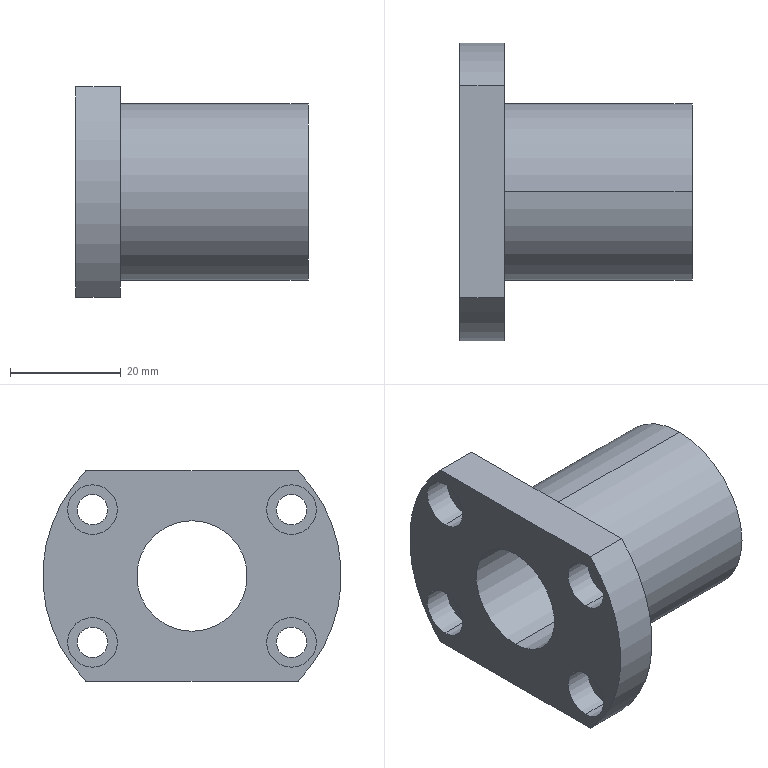Part | SolidWorks | features BaseBody 1 | 1 solid | 31 faces | box 42 x 54 x 38 mm | volume 27513 mm3 | cylinder 22 | plane 9 | commonest cylinder face diameters 5.5 x8 9 x8 20 x2 32 x2 54 x2
STEP:
#1=CARTESIAN_POINT('',(42.,0.,16.));
#2=VERTEX_POINT('',#1);
#3=CARTESIAN_POINT('',(42.,0.,-16.));
#4=VERTEX_POINT('',#3);
#5=CARTESIAN_POINT('',(42.,0.,0.));
#6=DIRECTION('',(-1.,0.,0.));
#7=DIRECTION('',(0.,0.,1.));
#8=AXIS2_PLACEMENT_3D('',#5,#6,#7);
#9=CIRCLE('',#8,16.);
#10=EDGE_CURVE('',#2,#4,#9,.T.);
#11=ORIENTED_EDGE('',*,*,#10,.T.);
#12=CARTESIAN_POINT('',(8.,0.,-16.));
#13=VERTEX_POINT('',#12);
#14=CARTESIAN_POINT('',(0.,0.,-16.));
#15=DIRECTION('',(-1.,0.,0.));
#16=VECTOR('',#15,1000.);
#17=LINE('',#14,#16);
#18=EDGE_CURVE('',#4,#13,#17,.T.);
#19=ORIENTED_EDGE('',*,*,#18,.T.);
#20=CARTESIAN_POINT('',(8.,0.,16.));
#21=VERTEX_POINT('',#20);
#22=CARTESIAN_POINT('',(8.,0.,0.));
#23=DIRECTION('',(1.,0.,0.));
#24=DIRECTION('',(0.,0.,1.));
#25=AXIS2_PLACEMENT_3D('',#22,#23,#24);
#26=CIRCLE('',#25,16.);
#27=EDGE_CURVE('',#13,#21,#26,.T.);
#28=ORIENTED_EDGE('',*,*,#27,.T.);
#29=CARTESIAN_POINT('',(0.,0.,16.));
#30=DIRECTION('',(-1.,0.,0.));
#31=VECTOR('',#30,1000.);
#32=LINE('',#29,#31);
#33=EDGE_CURVE('',#2,#21,#32,.T.);
#34=ORIENTED_EDGE('',*,*,#33,.F.);
#35=EDGE_LOOP('',(#11,#19,#28,#34));
#36=FACE_OUTER_BOUND('',#35,.T.);
#37=CARTESIAN_POINT('',(0.,0.,0.));
#38=DIRECTION('',(-1.,0.,0.));
#39=DIRECTION('',(0.,0.,1.));
#40=AXIS2_PLACEMENT_3D('',#37,#38,#39);
#41=CYLINDRICAL_SURFACE('',#40,16.);
#42=ADVANCED_FACE('',(#36),#41,.T.);
#43=CARTESIAN_POINT('',(8.,18.,14.75));
#44=VERTEX_POINT('',#43);
#45=CARTESIAN_POINT('',(8.,18.,9.25));
#46=VERTEX_POINT('',#45);
#47=CARTESIAN_POINT('',(8.,18.,12.));
#48=DIRECTION('',(1.,0.,0.));
#49=DIRECTION('',(0.,0.,1.));
#50=AXIS2_PLACEMENT_3D('',#47,#48,#49);
#51=CIRCLE('',#50,2.75);
#52=EDGE_CURVE('',#44,#46,#51,.T.);
#53=ORIENTED_EDGE('',*,*,#52,.T.);
#54=CARTESIAN_POINT('',(5.1,18.,9.25));
#55=VERTEX_POINT('',#54);
#56=CARTESIAN_POINT('',(42.001,18.,9.25));
#57=DIRECTION('',(-1.,0.,0.));
#58=VECTOR('',#57,1000.);
#59=LINE('',#56,#58);
#60=EDGE_CURVE('',#46,#55,#59,.T.);
#61=ORIENTED_EDGE('',*,*,#60,.T.);
#62=CARTESIAN_POINT('',(5.1,18.,14.75));
#63=VERTEX_POINT('',#62);
#64=CARTESIAN_POINT('',(5.1,18.,12.));
#65=DIRECTION('',(1.,0.,0.));
#66=DIRECTION('',(0.,0.,1.));
#67=AXIS2_PLACEMENT_3D('',#64,#65,#66);
#68=CIRCLE('',#67,2.75);
#69=EDGE_CURVE('',#63,#55,#68,.T.);
#70=ORIENTED_EDGE('',*,*,#69,.F.);
#71=CARTESIAN_POINT('',(42.001,18.,14.75));
#72=DIRECTION('',(-1.,0.,0.));
#73=VECTOR('',#72,1000.);
#74=LINE('',#71,#73);
#75=EDGE_CURVE('',#44,#63,#74,.T.);
#76=ORIENTED_EDGE('',*,*,#75,.F.);
#77=EDGE_LOOP('',(#53,#61,#70,#76));
#78=FACE_OUTER_BOUND('',#77,.T.);
#79=CARTESIAN_POINT('',(42.001,18.,12.));
#80=DIRECTION('',(-1.,0.,0.));
#81=DIRECTION('',(0.,0.,1.));
#82=AXIS2_PLACEMENT_3D('',#79,#80,#81);
#83=CYLINDRICAL_SURFACE('',#82,2.75);
#84=ADVANCED_FACE('',(#78),#83,.F.);
#85=CARTESIAN_POINT('',(8.,18.,-9.25));
#86=VERTEX_POINT('',#85);
#87=CARTESIAN_POINT('',(8.,18.,-14.75));
#88=VERTEX_POINT('',#87);
#89=CARTESIAN_POINT('',(8.,18.,-12.));
#90=DIRECTION('',(1.,0.,0.));
#91=DIRECTION('',(0.,0.,1.));
#92=AXIS2_PLACEMENT_3D('',#89,#90,#91);
#93=CIRCLE('',#92,2.75);
#94=EDGE_CURVE('',#86,#88,#93,.T.);
#95=ORIENTED_EDGE('',*,*,#94,.T.);
#96=CARTESIAN_POINT('',(5.1,18.,-14.75));
#97=VERTEX_POINT('',#96);
#98=CARTESIAN_POINT('',(42.001,18.,-14.75));
#99=DIRECTION('',(-1.,0.,0.));
#100=VECTOR('',#99,1000.);
#101=LINE('',#98,#100);
#102=EDGE_CURVE('',#88,#97,#101,.T.);
#103=ORIENTED_EDGE('',*,*,#102,.T.);
#104=CARTESIAN_POINT('',(5.1,18.,-9.25));
#105=VERTEX_POINT('',#104);
#106=CARTESIAN_POINT('',(5.1,18.,-12.));
#107=DIRECTION('',(1.,0.,0.));
#108=DIRECTION('',(0.,0.,1.));
#109=AXIS2_PLACEMENT_3D('',#106,#107,#108);
#110=CIRCLE('',#109,2.75);
#111=EDGE_CURVE('',#105,#97,#110,.T.);
#112=ORIENTED_EDGE('',*,*,#111,.F.);
#113=CARTESIAN_POINT('',(42.001,18.,-9.25));
#114=DIRECTION('',(-1.,0.,0.));
#115=VECTOR('',#114,1000.);
#116=LINE('',#113,#115);
#117=EDGE_CURVE('',#86,#105,#116,.T.);
#118=ORIENTED_EDGE('',*,*,#117,.F.);
#119=EDGE_LOOP('',(#95,#103,#112,#118));
#120=FACE_OUTER_BOUND('',#119,.T.);
#121=CARTESIAN_POINT('',(42.001,18.,-12.));
#122=DIRECTION('',(-1.,0.,0.));
#123=DIRECTION('',(0.,0.,1.));
#124=AXIS2_PLACEMENT_3D('',#121,#122,#123);
#125=CYLINDRICAL_SURFACE('',#124,2.75);
#126=ADVANCED_FACE('',(#120),#125,.F.);
#127=CARTESIAN_POINT('',(8.,-18.,-9.25));
#128=VERTEX_POINT('',#127);
#129=CARTESIAN_POINT('',(8.,-18.,-14.75));
#130=VERTEX_POINT('',#129);
#131=CARTESIAN_POINT('',(8.,-18.,-12.));
#132=DIRECTION('',(1.,0.,0.));
#133=DIRECTION('',(0.,0.,1.));
#134=AXIS2_PLACEMENT_3D('',#131,#132,#133);
#135=CIRCLE('',#134,2.75);
#136=EDGE_CURVE('',#128,#130,#135,.T.);
#137=ORIENTED_EDGE('',*,*,#136,.T.);
#138=CARTESIAN_POINT('',(5.1,-18.,-14.75));
#139=VERTEX_POINT('',#138);
#140=CARTESIAN_POINT('',(42.001,-18.,-14.75));
#141=DIRECTION('',(-1.,0.,0.));
#142=VECTOR('',#141,1000.);
#143=LINE('',#140,#142);
#144=EDGE_CURVE('',#130,#139,#143,.T.);
#145=ORIENTED_EDGE('',*,*,#144,.T.);
#146=CARTESIAN_POINT('',(5.1,-18.,-9.25));
#147=VERTEX_POINT('',#146);
#148=CARTESIAN_POINT('',(5.1,-18.,-12.));
#149=DIRECTION('',(1.,0.,0.));
#150=DIRECTION('',(0.,0.,1.));
#151=AXIS2_PLACEMENT_3D('',#148,#149,#150);
#152=CIRCLE('',#151,2.75);
#153=EDGE_CURVE('',#147,#139,#152,.T.);
#154=ORIENTED_EDGE('',*,*,#153,.F.);
#155=CARTESIAN_POINT('',(42.001,-18.,-9.25));
#156=DIRECTION('',(-1.,0.,0.));
#157=VECTOR('',#156,1000.);
#158=LINE('',#155,#157);
#159=EDGE_CURVE('',#128,#147,#158,.T.);
#160=ORIENTED_EDGE('',*,*,#159,.F.);
#161=EDGE_LOOP('',(#137,#145,#154,#160));
#162=FACE_OUTER_BOUND('',#161,.T.);
#163=CARTESIAN_POINT('',(42.001,-18.,-12.));
#164=DIRECTION('',(-1.,0.,0.));
#165=DIRECTION('',(0.,0.,1.));
#166=AXIS2_PLACEMENT_3D('',#163,#164,#165);
#167=CYLINDRICAL_SURFACE('',#166,2.75);
#168=ADVANCED_FACE('',(#162),#167,.F.);
#169=CARTESIAN_POINT('',(8.,-18.,14.75));
#170=VERTEX_POINT('',#169);
#171=CARTESIAN_POINT('',(8.,-18.,9.25));
#172=VERTEX_POINT('',#171);
#173=CARTESIAN_POINT('',(8.,-18.,12.));
#174=DIRECTION('',(1.,0.,0.));
#175=DIRECTION('',(0.,0.,1.));
#176=AXIS2_PLACEMENT_3D('',#173,#174,#175);
#177=CIRCLE('',#176,2.75);
#178=EDGE_CURVE('',#170,#172,#177,.T.);
#179=ORIENTED_EDGE('',*,*,#178,.T.);
#180=CARTESIAN_POINT('',(5.1,-18.,9.25));
#181=VERTEX_POINT('',#180);
#182=CARTESIAN_POINT('',(42.001,-18.,9.25));
#183=DIRECTION('',(-1.,0.,0.));
#184=VECTOR('',#183,1000.);
#185=LINE('',#182,#184);
#186=EDGE_CURVE('',#172,#181,#185,.T.);
#187=ORIENTED_EDGE('',*,*,#186,.T.);
#188=CARTESIAN_POINT('',(5.1,-18.,14.75));
#189=VERTEX_POINT('',#188);
#190=CARTESIAN_POINT('',(5.1,-18.,12.));
#191=DIRECTION('',(1.,0.,0.));
#192=DIRECTION('',(0.,0.,1.));
#193=AXIS2_PLACEMENT_3D('',#190,#191,#192);
#194=CIRCLE('',#193,2.75);
#195=EDGE_CURVE('',#189,#181,#194,.T.);
#196=ORIENTED_EDGE('',*,*,#195,.F.);
#197=CARTESIAN_POINT('',(42.001,-18.,14.75));
#198=DIRECTION('',(-1.,0.,0.));
#199=VECTOR('',#198,1000.);
#200=LINE('',#197,#199);
#201=EDGE_CURVE('',#170,#189,#200,.T.);
#202=ORIENTED_EDGE('',*,*,#201,.F.);
#203=EDGE_LOOP('',(#179,#187,#196,#202));
#204=FACE_OUTER_BOUND('',#203,.T.);
#205=CARTESIAN_POINT('',(42.001,-18.,12.));
#206=DIRECTION('',(-1.,0.,0.));
#207=DIRECTION('',(0.,0.,1.));
#208=AXIS2_PLACEMENT_3D('',#205,#206,#207);
#209=CYLINDRICAL_SURFACE('',#208,2.75);
#210=ADVANCED_FACE('',(#204),#209,.F.);
#211=CARTESIAN_POINT('',(42.,0.,10.));
#212=VERTEX_POINT('',#211);
#213=CARTESIAN_POINT('',(42.,0.,-10.));
#214=VERTEX_POINT('',#213);
#215=CARTESIAN_POINT('',(42.,0.,0.));
#216=DIRECTION('',(1.,0.,0.));
#217=DIRECTION('',(0.,0.,1.));
#218=AXIS2_PLACEMENT_3D('',#215,#216,#217);
#219=CIRCLE('',#218,10.);
#220=EDGE_CURVE('',#212,#214,#219,.T.);
#221=ORIENTED_EDGE('',*,*,#220,.T.);
#222=CARTESIAN_POINT('',(0.,0.,-10.));
#223=VERTEX_POINT('',#222);
#224=CARTESIAN_POINT('',(0.,0.,-10.));
#225=DIRECTION('',(-1.,0.,0.));
#226=VECTOR('',#225,1000.);
#227=LINE('',#224,#226);
#228=EDGE_CURVE('',#214,#223,#227,.T.);
#229=ORIENTED_EDGE('',*,*,#228,.T.);
#230=CARTESIAN_POINT('',(0.,0.,10.));
#231=VERTEX_POINT('',#230);
#232=CARTESIAN_POINT('',(0.,0.,0.));
#233=DIRECTION('',(1.,0.,0.));
#234=DIRECTION('',(0.,0.,1.));
#235=AXIS2_PLACEMENT_3D('',#232,#233,#234);
#236=CIRCLE('',#235,10.);
#237=EDGE_CURVE('',#231,#223,#236,.T.);
#238=ORIENTED_EDGE('',*,*,#237,.F.);
#239=CARTESIAN_POINT('',(0.,0.,10.));
#240=DIRECTION('',(-1.,0.,0.));
#241=VECTOR('',#240,1000.);
#242=LINE('',#239,#241);
#243=EDGE_CURVE('',#212,#231,#242,.T.);
#244=ORIENTED_EDGE('',*,*,#243,.F.);
#245=EDGE_LOOP('',(#221,#229,#238,#244));
#246=FACE_OUTER_BOUND('',#245,.T.);
#247=CARTESIAN_POINT('',(0.,0.,0.));
#248=DIRECTION('',(-1.,0.,0.));
#249=DIRECTION('',(0.,0.,1.));
#250=AXIS2_PLACEMENT_3D('',#247,#248,#249);
#251=CYLINDRICAL_SURFACE('',#250,10.);
#252=ADVANCED_FACE('',(#246),#251,.F.);
#253=CARTESIAN_POINT('',(5.1,18.,7.5));
#254=VERTEX_POINT('',#253);
#255=CARTESIAN_POINT('',(5.1,18.,16.5));
#256=VERTEX_POINT('',#255);
#257=CARTESIAN_POINT('',(5.1,18.,12.));
#258=DIRECTION('',(-1.,0.,0.));
#259=DIRECTION('',(0.,0.,1.));
#260=AXIS2_PLACEMENT_3D('',#257,#258,#259);
#261=CIRCLE('',#260,4.5);
#262=EDGE_CURVE('',#254,#256,#261,.T.);
#263=ORIENTED_EDGE('',*,*,#262,.F.);
#264=CARTESIAN_POINT('',(0.,18.,7.5));
#265=VERTEX_POINT('',#264);
#266=CARTESIAN_POINT('',(5.1,18.,7.5));
#267=DIRECTION('',(-1.,0.,0.));
#268=VECTOR('',#267,1000.);
#269=LINE('',#266,#268);
#270=EDGE_CURVE('',#254,#265,#269,.T.);
#271=ORIENTED_EDGE('',*,*,#270,.T.);
#272=CARTESIAN_POINT('',(0.,18.,16.5));
#273=VERTEX_POINT('',#272);
#274=CARTESIAN_POINT('',(0.,18.,12.));
#275=DIRECTION('',(-1.,0.,0.));
#276=DIRECTION('',(0.,0.,1.));
#277=AXIS2_PLACEMENT_3D('',#274,#275,#276);
#278=CIRCLE('',#277,4.5);
#279=EDGE_CURVE('',#265,#273,#278,.T.);
#280=ORIENTED_EDGE('',*,*,#279,.T.);
#281=CARTESIAN_POINT('',(5.1,18.,16.5));
#282=DIRECTION('',(-1.,0.,0.));
#283=VECTOR('',#282,1000.);
#284=LINE('',#281,#283);
#285=EDGE_CURVE('',#256,#273,#284,.T.);
#286=ORIENTED_EDGE('',*,*,#285,.F.);
#287=EDGE_LOOP('',(#263,#271,#280,#286));
#288=FACE_OUTER_BOUND('',#287,.T.);
#289=CARTESIAN_POINT('',(5.1,18.,12.));
#290=DIRECTION('',(-1.,0.,0.));
#291=DIRECTION('',(0.,0.,1.));
#292=AXIS2_PLACEMENT_3D('',#289,#290,#291);
#293=CYLINDRICAL_SURFACE('',#292,4.5);
#294=ADVANCED_FACE('',(#288),#293,.F.);
#295=CARTESIAN_POINT('',(5.1,18.,-16.5));
#296=VERTEX_POINT('',#295);
#297=CARTESIAN_POINT('',(5.1,18.,-7.5));
#298=VERTEX_POINT('',#297);
#299=CARTESIAN_POINT('',(5.1,18.,-12.));
#300=DIRECTION('',(-1.,0.,0.));
#301=DIRECTION('',(0.,0.,1.));
#302=AXIS2_PLACEMENT_3D('',#299,#300,#301);
#303=CIRCLE('',#302,4.5);
#304=EDGE_CURVE('',#296,#298,#303,.T.);
#305=ORIENTED_EDGE('',*,*,#304,.F.);
#306=CARTESIAN_POINT('',(0.,18.,-16.5));
#307=VERTEX_POINT('',#306);
#308=CARTESIAN_POINT('',(5.1,18.,-16.5));
#309=DIRECTION('',(-1.,0.,0.));
#310=VECTOR('',#309,1000.);
#311=LINE('',#308,#310);
#312=EDGE_CURVE('',#296,#307,#311,.T.);
#313=ORIENTED_EDGE('',*,*,#312,.T.);
#314=CARTESIAN_POINT('',(0.,18.,-7.5));
#315=VERTEX_POINT('',#314);
#316=CARTESIAN_POINT('',(0.,18.,-12.));
#317=DIRECTION('',(-1.,0.,0.));
#318=DIRECTION('',(0.,0.,1.));
#319=AXIS2_PLACEMENT_3D('',#316,#317,#318);
#320=CIRCLE('',#319,4.5);
#321=EDGE_CURVE('',#307,#315,#320,.T.);
#322=ORIENTED_EDGE('',*,*,#321,.T.);
#323=CARTESIAN_POINT('',(5.1,18.,-7.5));
#324=DIRECTION('',(-1.,0.,0.));
#325=VECTOR('',#324,1000.);
#326=LINE('',#323,#325);
#327=EDGE_CURVE('',#298,#315,#326,.T.);
#328=ORIENTED_EDGE('',*,*,#327,.F.);
#329=EDGE_LOOP('',(#305,#313,#322,#328));
#330=FACE_OUTER_BOUND('',#329,.T.);
#331=CARTESIAN_POINT('',(5.1,18.,-12.));
#332=DIRECTION('',(-1.,0.,0.));
#333=DIRECTION('',(0.,0.,1.));
#334=AXIS2_PLACEMENT_3D('',#331,#332,#333);
#335=CYLINDRICAL_SURFACE('',#334,4.5);
#336=ADVANCED_FACE('',(#330),#335,.F.);
#337=CARTESIAN_POINT('',(5.1,-18.,-16.5));
#338=VERTEX_POINT('',#337);
#339=CARTESIAN_POINT('',(5.1,-18.,-7.5));
#340=VERTEX_POINT('',#339);
#341=CARTESIAN_POINT('',(5.1,-18.,-12.));
#342=DIRECTION('',(-1.,0.,0.));
#343=DIRECTION('',(0.,0.,1.));
#344=AXIS2_PLACEMENT_3D('',#341,#342,#343);
#345=CIRCLE('',#344,4.5);
#346=EDGE_CURVE('',#338,#340,#345,.T.);
#347=ORIENTED_EDGE('',*,*,#346,.F.);
#348=CARTESIAN_POINT('',(0.,-18.,-16.5));
#349=VERTEX_POINT('',#348);
#350=CARTESIAN_POINT('',(5.1,-18.,-16.5));
#351=DIRECTION('',(-1.,0.,0.));
#352=VECTOR('',#351,1000.);
#353=LINE('',#350,#352);
#354=EDGE_CURVE('',#338,#349,#353,.T.);
#355=ORIENTED_EDGE('',*,*,#354,.T.);
#356=CARTESIAN_POINT('',(0.,-18.,-7.5));
#357=VERTEX_POINT('',#356);
#358=CARTESIAN_POINT('',(0.,-18.,-12.));
#359=DIRECTION('',(-1.,0.,0.));
#360=DIRECTION('',(0.,0.,1.));
#361=AXIS2_PLACEMENT_3D('',#358,#359,#360);
#362=CIRCLE('',#361,4.5);
#363=EDGE_CURVE('',#349,#357,#362,.T.);
#364=ORIENTED_EDGE('',*,*,#363,.T.);
#365=CARTESIAN_POINT('',(5.1,-18.,-7.5));
#366=DIRECTION('',(-1.,0.,0.));
#367=VECTOR('',#366,1000.);
#368=LINE('',#365,#367);
#369=EDGE_CURVE('',#340,#357,#368,.T.);
#370=ORIENTED_EDGE('',*,*,#369,.F.);
#371=EDGE_LOOP('',(#347,#355,#364,#370));
#372=FACE_OUTER_BOUND('',#371,.T.);
#373=CARTESIAN_POINT('',(5.1,-18.,-12.));
#374=DIRECTION('',(-1.,0.,0.));
#375=DIRECTION('',(0.,0.,1.));
#376=AXIS2_PLACEMENT_3D('',#373,#374,#375);
#377=CYLINDRICAL_SURFACE('',#376,4.5);
#378=ADVANCED_FACE('',(#372),#377,.F.);
#379=CARTESIAN_POINT('',(5.1,-18.,7.5));
#380=VERTEX_POINT('',#379);
#381=CARTESIAN_POINT('',(5.1,-18.,16.5));
#382=VERTEX_POINT('',#381);
#383=CARTESIAN_POINT('',(5.1,-18.,12.));
#384=DIRECTION('',(-1.,0.,0.));
#385=DIRECTION('',(0.,0.,1.));
#386=AXIS2_PLACEMENT_3D('',#383,#384,#385);
#387=CIRCLE('',#386,4.5);
#388=EDGE_CURVE('',#380,#382,#387,.T.);
#389=ORIENTED_EDGE('',*,*,#388,.F.);
#390=CARTESIAN_POINT('',(0.,-18.,7.5));
#391=VERTEX_POINT('',#390);
#392=CARTESIAN_POINT('',(5.1,-18.,7.5));
#393=DIRECTION('',(-1.,0.,0.));
#394=VECTOR('',#393,1000.);
#395=LINE('',#392,#394);
#396=EDGE_CURVE('',#380,#391,#395,.T.);
#397=ORIENTED_EDGE('',*,*,#396,.T.);
#398=CARTESIAN_POINT('',(0.,-18.,16.5));
#399=VERTEX_POINT('',#398);
#400=CARTESIAN_POINT('',(0.,-18.,12.));
#401=DIRECTION('',(-1.,0.,0.));
#402=DIRECTION('',(0.,0.,1.));
#403=AXIS2_PLACEMENT_3D('',#400,#401,#402);
#404=CIRCLE('',#403,4.5);
#405=EDGE_CURVE('',#391,#399,#404,.T.);
#406=ORIENTED_EDGE('',*,*,#405,.T.);
#407=CARTESIAN_POINT('',(5.1,-18.,16.5));
#408=DIRECTION('',(-1.,0.,0.));
#409=VECTOR('',#408,1000.);
#410=LINE('',#407,#409);
#411=EDGE_CURVE('',#382,#399,#410,.T.);
#412=ORIENTED_EDGE('',*,*,#411,.F.);
#413=EDGE_LOOP('',(#389,#397,#406,#412));
#414=FACE_OUTER_BOUND('',#413,.T.);
#415=CARTESIAN_POINT('',(5.1,-18.,12.));
#416=DIRECTION('',(-1.,0.,0.));
#417=DIRECTION('',(0.,0.,1.));
#418=AXIS2_PLACEMENT_3D('',#415,#416,#417);
#419=CYLINDRICAL_SURFACE('',#418,4.5);
#420=ADVANCED_FACE('',(#414),#419,.F.);
#421=ORIENTED_EDGE('',*,*,#18,.F.);
#422=CARTESIAN_POINT('',(42.,0.,0.));
#423=DIRECTION('',(-1.,0.,0.));
#424=DIRECTION('',(0.,0.,1.));
#425=AXIS2_PLACEMENT_3D('',#422,#423,#424);
#426=CIRCLE('',#425,16.);
#427=EDGE_CURVE('',#4,#2,#426,.T.);
#428=ORIENTED_EDGE('',*,*,#427,.T.);
#429=ORIENTED_EDGE('',*,*,#33,.T.);
#430=CARTESIAN_POINT('',(8.,0.,0.));
#431=DIRECTION('',(1.,0.,0.));
#432=DIRECTION('',(0.,0.,1.));
#433=AXIS2_PLACEMENT_3D('',#430,#431,#432);
#434=CIRCLE('',#433,16.);
#435=EDGE_CURVE('',#21,#13,#434,.T.);
#436=ORIENTED_EDGE('',*,*,#435,.T.);
#437=EDGE_LOOP('',(#421,#428,#429,#436));
#438=FACE_OUTER_BOUND('',#437,.T.);
#439=CARTESIAN_POINT('',(0.,0.,0.));
#440=DIRECTION('',(-1.,0.,0.));
#441=DIRECTION('',(0.,0.,1.));
#442=AXIS2_PLACEMENT_3D('',#439,#440,#441);
#443=CYLINDRICAL_SURFACE('',#442,16.);
#444=ADVANCED_FACE('',(#438),#443,.T.);
#445=ORIENTED_EDGE('',*,*,#435,.F.);
#446=ORIENTED_EDGE('',*,*,#27,.F.);
#447=EDGE_LOOP('',(#445,#446));
#448=FACE_BOUND('',#447,.T.);
#449=CARTESIAN_POINT('',(8.,-19.183,19.));
#450=VERTEX_POINT('',#449);
#451=CARTESIAN_POINT('',(8.,19.183,19.));
#452=VERTEX_POINT('',#451);
#453=CARTESIAN_POINT('',(8.,27.,19.));
#454=DIRECTION('',(0.,1.,0.));
#455=VECTOR('',#454,1000.);
#456=LINE('',#453,#455);
#457=EDGE_CURVE('',#450,#452,#456,.T.);
#458=ORIENTED_EDGE('',*,*,#457,.F.);
#459=CARTESIAN_POINT('',(8.,-19.183,-19.));
#460=VERTEX_POINT('',#459);
#461=CARTESIAN_POINT('',(8.,0.,0.));
#462=DIRECTION('',(-1.,0.,0.));
#463=DIRECTION('',(0.,0.,1.));
#464=AXIS2_PLACEMENT_3D('',#461,#462,#463);
#465=CIRCLE('',#464,27.);
#466=EDGE_CURVE('',#460,#450,#465,.T.);
#467=ORIENTED_EDGE('',*,*,#466,.F.);
#468=CARTESIAN_POINT('',(8.,19.183,-19.));
#469=VERTEX_POINT('',#468);
#470=CARTESIAN_POINT('',(8.,27.,-19.));
#471=DIRECTION('',(0.,-1.,0.));
#472=VECTOR('',#471,1000.);
#473=LINE('',#470,#472);
#474=EDGE_CURVE('',#469,#460,#473,.T.);
#475=ORIENTED_EDGE('',*,*,#474,.F.);
#476=CARTESIAN_POINT('',(8.,0.,0.));
#477=DIRECTION('',(-1.,0.,0.));
#478=DIRECTION('',(0.,0.,1.));
#479=AXIS2_PLACEMENT_3D('',#476,#477,#478);
#480=CIRCLE('',#479,27.);
#481=EDGE_CURVE('',#452,#469,#480,.T.);
#482=ORIENTED_EDGE('',*,*,#481,.F.);
#483=EDGE_LOOP('',(#458,#467,#475,#482));
#484=FACE_OUTER_BOUND('',#483,.T.);
#485=ORIENTED_EDGE('',*,*,#52,.F.);
#486=CARTESIAN_POINT('',(8.,18.,12.));
#487=DIRECTION('',(1.,0.,0.));
#488=DIRECTION('',(0.,0.,1.));
#489=AXIS2_PLACEMENT_3D('',#486,#487,#488);
#490=CIRCLE('',#489,2.75);
#491=EDGE_CURVE('',#46,#44,#490,.T.);
#492=ORIENTED_EDGE('',*,*,#491,.F.);
#493=EDGE_LOOP('',(#485,#492));
#494=FACE_BOUND('',#493,.T.);
#495=ORIENTED_EDGE('',*,*,#94,.F.);
#496=CARTESIAN_POINT('',(8.,18.,-12.));
#497=DIRECTION('',(1.,0.,0.));
#498=DIRECTION('',(0.,0.,1.));
#499=AXIS2_PLACEMENT_3D('',#496,#497,#498);
#500=CIRCLE('',#499,2.75);
#501=EDGE_CURVE('',#88,#86,#500,.T.);
#502=ORIENTED_EDGE('',*,*,#501,.F.);
#503=EDGE_LOOP('',(#495,#502));
#504=FACE_BOUND('',#503,.T.);
#505=ORIENTED_EDGE('',*,*,#136,.F.);
#506=CARTESIAN_POINT('',(8.,-18.,-12.));
#507=DIRECTION('',(1.,0.,0.));
#508=DIRECTION('',(0.,0.,1.));
#509=AXIS2_PLACEMENT_3D('',#506,#507,#508);
#510=CIRCLE('',#509,2.75);
#511=EDGE_CURVE('',#130,#128,#510,.T.);
#512=ORIENTED_EDGE('',*,*,#511,.F.);
#513=EDGE_LOOP('',(#505,#512));
#514=FACE_BOUND('',#513,.T.);
#515=ORIENTED_EDGE('',*,*,#178,.F.);
#516=CARTESIAN_POINT('',(8.,-18.,12.));
#517=DIRECTION('',(1.,0.,0.));
#518=DIRECTION('',(0.,0.,1.));
#519=AXIS2_PLACEMENT_3D('',#516,#517,#518);
#520=CIRCLE('',#519,2.75);
#521=EDGE_CURVE('',#172,#170,#520,.T.);
#522=ORIENTED_EDGE('',*,*,#521,.F.);
#523=EDGE_LOOP('',(#515,#522));
#524=FACE_BOUND('',#523,.T.);
#525=CARTESIAN_POINT('',(8.,27.,0.));
#526=DIRECTION('',(-1.,0.,0.));
#527=DIRECTION('',(0.,0.,1.));
#528=AXIS2_PLACEMENT_3D('',#525,#526,#527);
#529=PLANE('',#528);
#530=ADVANCED_FACE('',(#448,#484,#494,#504,#514,#524),#529,.F.);
#531=ORIENTED_EDGE('',*,*,#220,.F.);
#532=CARTESIAN_POINT('',(42.,0.,0.));
#533=DIRECTION('',(1.,0.,0.));
#534=DIRECTION('',(0.,0.,1.));
#535=AXIS2_PLACEMENT_3D('',#532,#533,#534);
#536=CIRCLE('',#535,10.);
#537=EDGE_CURVE('',#214,#212,#536,.T.);
#538=ORIENTED_EDGE('',*,*,#537,.F.);
#539=EDGE_LOOP('',(#531,#538));
#540=FACE_BOUND('',#539,.T.);
#541=ORIENTED_EDGE('',*,*,#10,.F.);
#542=ORIENTED_EDGE('',*,*,#427,.F.);
#543=EDGE_LOOP('',(#541,#542));
#544=FACE_OUTER_BOUND('',#543,.T.);
#545=CARTESIAN_POINT('',(42.,16.,0.));
#546=DIRECTION('',(-1.,0.,0.));
#547=DIRECTION('',(0.,0.,1.));
#548=AXIS2_PLACEMENT_3D('',#545,#546,#547);
#549=PLANE('',#548);
#550=ADVANCED_FACE('',(#540,#544),#549,.F.);
#551=ORIENTED_EDGE('',*,*,#481,.T.);
#552=CARTESIAN_POINT('',(0.,19.183,-19.));
#553=VERTEX_POINT('',#552);
#554=CARTESIAN_POINT('',(0.,19.183,-19.));
#555=DIRECTION('',(-1.,0.,0.));
#556=VECTOR('',#555,1000.);
#557=LINE('',#554,#556);
#558=EDGE_CURVE('',#469,#553,#557,.T.);
#559=ORIENTED_EDGE('',*,*,#558,.T.);
#560=CARTESIAN_POINT('',(0.,19.183,19.));
#561=VERTEX_POINT('',#560);
#562=CARTESIAN_POINT('',(0.,0.,0.));
#563=DIRECTION('',(1.,0.,0.));
#564=DIRECTION('',(0.,0.,1.));
#565=AXIS2_PLACEMENT_3D('',#562,#563,#564);
#566=CIRCLE('',#565,27.);
#567=EDGE_CURVE('',#553,#561,#566,.T.);
#568=ORIENTED_EDGE('',*,*,#567,.T.);
#569=CARTESIAN_POINT('',(0.,19.183,19.));
#570=DIRECTION('',(1.,0.,0.));
#571=VECTOR('',#570,1000.);
#572=LINE('',#569,#571);
#573=EDGE_CURVE('',#561,#452,#572,.T.);
#574=ORIENTED_EDGE('',*,*,#573,.T.);
#575=EDGE_LOOP('',(#551,#559,#568,#574));
#576=FACE_OUTER_BOUND('',#575,.T.);
#577=CARTESIAN_POINT('',(0.,0.,0.));
#578=DIRECTION('',(-1.,0.,0.));
#579=DIRECTION('',(0.,0.,1.));
#580=AXIS2_PLACEMENT_3D('',#577,#578,#579);
#581=CYLINDRICAL_SURFACE('',#580,27.);
#582=ADVANCED_FACE('',(#576),#581,.T.);
#583=ORIENTED_EDGE('',*,*,#573,.F.);
#584=CARTESIAN_POINT('',(0.,-19.183,19.));
#585=VERTEX_POINT('',#584);
#586=CARTESIAN_POINT('',(0.,19.183,19.));
#587=DIRECTION('',(0.,1.,0.));
#588=VECTOR('',#587,1000.);
#589=LINE('',#586,#588);
#590=EDGE_CURVE('',#585,#561,#589,.T.);
#591=ORIENTED_EDGE('',*,*,#590,.F.);
#592=CARTESIAN_POINT('',(42.001,-19.183,19.));
#593=DIRECTION('',(-1.,0.,0.));
#594=VECTOR('',#593,1000.);
#595=LINE('',#592,#594);
#596=EDGE_CURVE('',#450,#585,#595,.T.);
#597=ORIENTED_EDGE('',*,*,#596,.F.);
#598=ORIENTED_EDGE('',*,*,#457,.T.);
#599=EDGE_LOOP('',(#583,#591,#597,#598));
#600=FACE_OUTER_BOUND('',#599,.T.);
#601=CARTESIAN_POINT('',(42.001,19.183,19.));
#602=DIRECTION('',(0.,0.,-1.));
#603=DIRECTION('',(-1.,0.,0.));
#604=AXIS2_PLACEMENT_3D('',#601,#602,#603);
#605=PLANE('',#604);
#606=ADVANCED_FACE('',(#600),#605,.F.);
#607=CARTESIAN_POINT('',(0.,-19.183,-19.));
#608=VERTEX_POINT('',#607);
#609=CARTESIAN_POINT('',(0.,0.,0.));
#610=DIRECTION('',(1.,0.,0.));
#611=DIRECTION('',(0.,0.,1.));
#612=AXIS2_PLACEMENT_3D('',#609,#610,#611);
#613=CIRCLE('',#612,27.);
#614=EDGE_CURVE('',#585,#608,#613,.T.);
#615=ORIENTED_EDGE('',*,*,#614,.T.);
#616=CARTESIAN_POINT('',(0.,-19.183,-19.));
#617=DIRECTION('',(1.,0.,0.));
#618=VECTOR('',#617,1000.);
#619=LINE('',#616,#618);
#620=EDGE_CURVE('',#608,#460,#619,.T.);
#621=ORIENTED_EDGE('',*,*,#620,.T.);
#622=ORIENTED_EDGE('',*,*,#466,.T.);
#623=ORIENTED_EDGE('',*,*,#596,.T.);
#624=EDGE_LOOP('',(#615,#621,#622,#623));
#625=FACE_OUTER_BOUND('',#624,.T.);
#626=CARTESIAN_POINT('',(0.,0.,0.));
#627=DIRECTION('',(-1.,0.,0.));
#628=DIRECTION('',(0.,0.,1.));
#629=AXIS2_PLACEMENT_3D('',#626,#627,#628);
#630=CYLINDRICAL_SURFACE('',#629,27.);
#631=ADVANCED_FACE('',(#625),#630,.T.);
#632=ORIENTED_EDGE('',*,*,#620,.F.);
#633=CARTESIAN_POINT('',(0.,19.183,-19.));
#634=DIRECTION('',(0.,-1.,0.));
#635=VECTOR('',#634,1000.);
#636=LINE('',#633,#635);
#637=EDGE_CURVE('',#553,#608,#636,.T.);
#638=ORIENTED_EDGE('',*,*,#637,.F.);
#639=ORIENTED_EDGE('',*,*,#558,.F.);
#640=ORIENTED_EDGE('',*,*,#474,.T.);
#641=EDGE_LOOP('',(#632,#638,#639,#640));
#642=FACE_OUTER_BOUND('',#641,.T.);
#643=CARTESIAN_POINT('',(42.001,19.183,-19.));
#644=DIRECTION('',(0.,0.,1.));
#645=DIRECTION('',(1.,0.,0.));
#646=AXIS2_PLACEMENT_3D('',#643,#644,#645);
#647=PLANE('',#646);
#648=ADVANCED_FACE('',(#642),#647,.F.);
#649=ORIENTED_EDGE('',*,*,#60,.F.);
#650=ORIENTED_EDGE('',*,*,#491,.T.);
#651=ORIENTED_EDGE('',*,*,#75,.T.);
#652=CARTESIAN_POINT('',(5.1,18.,12.));
#653=DIRECTION('',(1.,0.,0.));
#654=DIRECTION('',(0.,0.,1.));
#655=AXIS2_PLACEMENT_3D('',#652,#653,#654);
#656=CIRCLE('',#655,2.75);
#657=EDGE_CURVE('',#55,#63,#656,.T.);
#658=ORIENTED_EDGE('',*,*,#657,.F.);
#659=EDGE_LOOP('',(#649,#650,#651,#658));
#660=FACE_OUTER_BOUND('',#659,.T.);
#661=CARTESIAN_POINT('',(42.001,18.,12.));
#662=DIRECTION('',(-1.,0.,0.));
#663=DIRECTION('',(0.,0.,1.));
#664=AXIS2_PLACEMENT_3D('',#661,#662,#663);
#665=CYLINDRICAL_SURFACE('',#664,2.75);
#666=ADVANCED_FACE('',(#660),#665,.F.);
#667=ORIENTED_EDGE('',*,*,#102,.F.);
#668=ORIENTED_EDGE('',*,*,#501,.T.);
#669=ORIENTED_EDGE('',*,*,#117,.T.);
#670=CARTESIAN_POINT('',(5.1,18.,-12.));
#671=DIRECTION('',(1.,0.,0.));
#672=DIRECTION('',(0.,0.,1.));
#673=AXIS2_PLACEMENT_3D('',#670,#671,#672);
#674=CIRCLE('',#673,2.75);
#675=EDGE_CURVE('',#97,#105,#674,.T.);
#676=ORIENTED_EDGE('',*,*,#675,.F.);
#677=EDGE_LOOP('',(#667,#668,#669,#676));
#678=FACE_OUTER_BOUND('',#677,.T.);
#679=CARTESIAN_POINT('',(42.001,18.,-12.));
#680=DIRECTION('',(-1.,0.,0.));
#681=DIRECTION('',(0.,0.,1.));
#682=AXIS2_PLACEMENT_3D('',#679,#680,#681);
#683=CYLINDRICAL_SURFACE('',#682,2.75);
#684=ADVANCED_FACE('',(#678),#683,.F.);
#685=ORIENTED_EDGE('',*,*,#144,.F.);
#686=ORIENTED_EDGE('',*,*,#511,.T.);
#687=ORIENTED_EDGE('',*,*,#159,.T.);
#688=CARTESIAN_POINT('',(5.1,-18.,-12.));
#689=DIRECTION('',(1.,0.,0.));
#690=DIRECTION('',(0.,0.,1.));
#691=AXIS2_PLACEMENT_3D('',#688,#689,#690);
#692=CIRCLE('',#691,2.75);
#693=EDGE_CURVE('',#139,#147,#692,.T.);
#694=ORIENTED_EDGE('',*,*,#693,.F.);
#695=EDGE_LOOP('',(#685,#686,#687,#694));
#696=FACE_OUTER_BOUND('',#695,.T.);
#697=CARTESIAN_POINT('',(42.001,-18.,-12.));
#698=DIRECTION('',(-1.,0.,0.));
#699=DIRECTION('',(0.,0.,1.));
#700=AXIS2_PLACEMENT_3D('',#697,#698,#699);
#701=CYLINDRICAL_SURFACE('',#700,2.75);
#702=ADVANCED_FACE('',(#696),#701,.F.);
#703=ORIENTED_EDGE('',*,*,#186,.F.);
#704=ORIENTED_EDGE('',*,*,#521,.T.);
#705=ORIENTED_EDGE('',*,*,#201,.T.);
#706=CARTESIAN_POINT('',(5.1,-18.,12.));
#707=DIRECTION('',(1.,0.,0.));
#708=DIRECTION('',(0.,0.,1.));
#709=AXIS2_PLACEMENT_3D('',#706,#707,#708);
#710=CIRCLE('',#709,2.75);
#711=EDGE_CURVE('',#181,#189,#710,.T.);
#712=ORIENTED_EDGE('',*,*,#711,.F.);
#713=EDGE_LOOP('',(#703,#704,#705,#712));
#714=FACE_OUTER_BOUND('',#713,.T.);
#715=CARTESIAN_POINT('',(42.001,-18.,12.));
#716=DIRECTION('',(-1.,0.,0.));
#717=DIRECTION('',(0.,0.,1.));
#718=AXIS2_PLACEMENT_3D('',#715,#716,#717);
#719=CYLINDRICAL_SURFACE('',#718,2.75);
#720=ADVANCED_FACE('',(#714),#719,.F.);
#721=ORIENTED_EDGE('',*,*,#228,.F.);
#722=ORIENTED_EDGE('',*,*,#537,.T.);
#723=ORIENTED_EDGE('',*,*,#243,.T.);
#724=CARTESIAN_POINT('',(0.,0.,0.));
#725=DIRECTION('',(1.,0.,0.));
#726=DIRECTION('',(0.,0.,1.));
#727=AXIS2_PLACEMENT_3D('',#724,#725,#726);
#728=CIRCLE('',#727,10.);
#729=EDGE_CURVE('',#223,#231,#728,.T.);
#730=ORIENTED_EDGE('',*,*,#729,.F.);
#731=EDGE_LOOP('',(#721,#722,#723,#730));
#732=FACE_OUTER_BOUND('',#731,.T.);
#733=CARTESIAN_POINT('',(0.,0.,0.));
#734=DIRECTION('',(-1.,0.,0.));
#735=DIRECTION('',(0.,0.,1.));
#736=AXIS2_PLACEMENT_3D('',#733,#734,#735);
#737=CYLINDRICAL_SURFACE('',#736,10.);
#738=ADVANCED_FACE('',(#732),#737,.F.);
#739=ORIENTED_EDGE('',*,*,#590,.T.);
#740=ORIENTED_EDGE('',*,*,#567,.F.);
#741=ORIENTED_EDGE('',*,*,#637,.T.);
#742=ORIENTED_EDGE('',*,*,#614,.F.);
#743=EDGE_LOOP('',(#739,#740,#741,#742));
#744=FACE_OUTER_BOUND('',#743,.T.);
#745=ORIENTED_EDGE('',*,*,#237,.T.);
#746=ORIENTED_EDGE('',*,*,#729,.T.);
#747=EDGE_LOOP('',(#745,#746));
#748=FACE_BOUND('',#747,.T.);
#749=CARTESIAN_POINT('',(0.,18.,12.));
#750=DIRECTION('',(-1.,0.,0.));
#751=DIRECTION('',(0.,0.,1.));
#752=AXIS2_PLACEMENT_3D('',#749,#750,#751);
#753=CIRCLE('',#752,4.5);
#754=EDGE_CURVE('',#273,#265,#753,.T.);
#755=ORIENTED_EDGE('',*,*,#754,.F.);
#756=ORIENTED_EDGE('',*,*,#279,.F.);
#757=EDGE_LOOP('',(#755,#756));
#758=FACE_BOUND('',#757,.T.);
#759=CARTESIAN_POINT('',(0.,18.,-12.));
#760=DIRECTION('',(-1.,0.,0.));
#761=DIRECTION('',(0.,0.,1.));
#762=AXIS2_PLACEMENT_3D('',#759,#760,#761);
#763=CIRCLE('',#762,4.5);
#764=EDGE_CURVE('',#315,#307,#763,.T.);
#765=ORIENTED_EDGE('',*,*,#764,.F.);
#766=ORIENTED_EDGE('',*,*,#321,.F.);
#767=EDGE_LOOP('',(#765,#766));
#768=FACE_BOUND('',#767,.T.);
#769=CARTESIAN_POINT('',(0.,-18.,-12.));
#770=DIRECTION('',(-1.,0.,0.));
#771=DIRECTION('',(0.,0.,1.));
#772=AXIS2_PLACEMENT_3D('',#769,#770,#771);
#773=CIRCLE('',#772,4.5);
#774=EDGE_CURVE('',#357,#349,#773,.T.);
#775=ORIENTED_EDGE('',*,*,#774,.F.);
#776=ORIENTED_EDGE('',*,*,#363,.F.);
#777=EDGE_LOOP('',(#775,#776));
#778=FACE_BOUND('',#777,.T.);
#779=CARTESIAN_POINT('',(0.,-18.,12.));
#780=DIRECTION('',(-1.,0.,0.));
#781=DIRECTION('',(0.,0.,1.));
#782=AXIS2_PLACEMENT_3D('',#779,#780,#781);
#783=CIRCLE('',#782,4.5);
#784=EDGE_CURVE('',#399,#391,#783,.T.);
#785=ORIENTED_EDGE('',*,*,#784,.F.);
#786=ORIENTED_EDGE('',*,*,#405,.F.);
#787=EDGE_LOOP('',(#785,#786));
#788=FACE_BOUND('',#787,.T.);
#789=CARTESIAN_POINT('',(0.,10.,0.));
#790=DIRECTION('',(1.,0.,0.));
#791=DIRECTION('',(0.,0.,-1.));
#792=AXIS2_PLACEMENT_3D('',#789,#790,#791);
#793=PLANE('',#792);
#794=ADVANCED_FACE('',(#744,#748,#758,#768,#778,#788),#793,.F.);
#795=ORIENTED_EDGE('',*,*,#69,.T.);
#796=ORIENTED_EDGE('',*,*,#657,.T.);
#797=EDGE_LOOP('',(#795,#796));
#798=FACE_BOUND('',#797,.T.);
#799=CARTESIAN_POINT('',(5.1,18.,12.));
#800=DIRECTION('',(-1.,0.,0.));
#801=DIRECTION('',(0.,0.,1.));
#802=AXIS2_PLACEMENT_3D('',#799,#800,#801);
#803=CIRCLE('',#802,4.5);
#804=EDGE_CURVE('',#256,#254,#803,.T.);
#805=ORIENTED_EDGE('',*,*,#804,.T.);
#806=ORIENTED_EDGE('',*,*,#262,.T.);
#807=EDGE_LOOP('',(#805,#806));
#808=FACE_OUTER_BOUND('',#807,.T.);
#809=CARTESIAN_POINT('',(5.1,18.,12.));
#810=DIRECTION('',(-1.,0.,0.));
#811=DIRECTION('',(0.,0.,1.));
#812=AXIS2_PLACEMENT_3D('',#809,#810,#811);
#813=PLANE('',#812);
#814=ADVANCED_FACE('',(#798,#808),#813,.T.);
#815=ORIENTED_EDGE('',*,*,#111,.T.);
#816=ORIENTED_EDGE('',*,*,#675,.T.);
#817=EDGE_LOOP('',(#815,#816));
#818=FACE_BOUND('',#817,.T.);
#819=CARTESIAN_POINT('',(5.1,18.,-12.));
#820=DIRECTION('',(-1.,0.,0.));
#821=DIRECTION('',(0.,0.,1.));
#822=AXIS2_PLACEMENT_3D('',#819,#820,#821);
#823=CIRCLE('',#822,4.5);
#824=EDGE_CURVE('',#298,#296,#823,.T.);
#825=ORIENTED_EDGE('',*,*,#824,.T.);
#826=ORIENTED_EDGE('',*,*,#304,.T.);
#827=EDGE_LOOP('',(#825,#826));
#828=FACE_OUTER_BOUND('',#827,.T.);
#829=CARTESIAN_POINT('',(5.1,18.,-12.));
#830=DIRECTION('',(-1.,0.,0.));
#831=DIRECTION('',(0.,0.,1.));
#832=AXIS2_PLACEMENT_3D('',#829,#830,#831);
#833=PLANE('',#832);
#834=ADVANCED_FACE('',(#818,#828),#833,.T.);
#835=ORIENTED_EDGE('',*,*,#153,.T.);
#836=ORIENTED_EDGE('',*,*,#693,.T.);
#837=EDGE_LOOP('',(#835,#836));
#838=FACE_BOUND('',#837,.T.);
#839=CARTESIAN_POINT('',(5.1,-18.,-12.));
#840=DIRECTION('',(-1.,0.,0.));
#841=DIRECTION('',(0.,0.,1.));
#842=AXIS2_PLACEMENT_3D('',#839,#840,#841);
#843=CIRCLE('',#842,4.5);
#844=EDGE_CURVE('',#340,#338,#843,.T.);
#845=ORIENTED_EDGE('',*,*,#844,.T.);
#846=ORIENTED_EDGE('',*,*,#346,.T.);
#847=EDGE_LOOP('',(#845,#846));
#848=FACE_OUTER_BOUND('',#847,.T.);
#849=CARTESIAN_POINT('',(5.1,-18.,-12.));
#850=DIRECTION('',(-1.,0.,0.));
#851=DIRECTION('',(0.,0.,1.));
#852=AXIS2_PLACEMENT_3D('',#849,#850,#851);
#853=PLANE('',#852);
#854=ADVANCED_FACE('',(#838,#848),#853,.T.);
#855=ORIENTED_EDGE('',*,*,#195,.T.);
#856=ORIENTED_EDGE('',*,*,#711,.T.);
#857=EDGE_LOOP('',(#855,#856));
#858=FACE_BOUND('',#857,.T.);
#859=CARTESIAN_POINT('',(5.1,-18.,12.));
#860=DIRECTION('',(-1.,0.,0.));
#861=DIRECTION('',(0.,0.,1.));
#862=AXIS2_PLACEMENT_3D('',#859,#860,#861);
#863=CIRCLE('',#862,4.5);
#864=EDGE_CURVE('',#382,#380,#863,.T.);
#865=ORIENTED_EDGE('',*,*,#864,.T.);
#866=ORIENTED_EDGE('',*,*,#388,.T.);
#867=EDGE_LOOP('',(#865,#866));
#868=FACE_OUTER_BOUND('',#867,.T.);
#869=CARTESIAN_POINT('',(5.1,-18.,12.));
#870=DIRECTION('',(-1.,0.,0.));
#871=DIRECTION('',(0.,0.,1.));
#872=AXIS2_PLACEMENT_3D('',#869,#870,#871);
#873=PLANE('',#872);
#874=ADVANCED_FACE('',(#858,#868),#873,.T.);
#875=ORIENTED_EDGE('',*,*,#270,.F.);
#876=ORIENTED_EDGE('',*,*,#804,.F.);
#877=ORIENTED_EDGE('',*,*,#285,.T.);
#878=ORIENTED_EDGE('',*,*,#754,.T.);
#879=EDGE_LOOP('',(#875,#876,#877,#878));
#880=FACE_OUTER_BOUND('',#879,.T.);
#881=CARTESIAN_POINT('',(5.1,18.,12.));
#882=DIRECTION('',(-1.,0.,0.));
#883=DIRECTION('',(0.,0.,1.));
#884=AXIS2_PLACEMENT_3D('',#881,#882,#883);
#885=CYLINDRICAL_SURFACE('',#884,4.5);
#886=ADVANCED_FACE('',(#880),#885,.F.);
#887=ORIENTED_EDGE('',*,*,#312,.F.);
#888=ORIENTED_EDGE('',*,*,#824,.F.);
#889=ORIENTED_EDGE('',*,*,#327,.T.);
#890=ORIENTED_EDGE('',*,*,#764,.T.);
#891=EDGE_LOOP('',(#887,#888,#889,#890));
#892=FACE_OUTER_BOUND('',#891,.T.);
#893=CARTESIAN_POINT('',(5.1,18.,-12.));
#894=DIRECTION('',(-1.,0.,0.));
#895=DIRECTION('',(0.,0.,1.));
#896=AXIS2_PLACEMENT_3D('',#893,#894,#895);
#897=CYLINDRICAL_SURFACE('',#896,4.5);
#898=ADVANCED_FACE('',(#892),#897,.F.);
#899=ORIENTED_EDGE('',*,*,#354,.F.);
#900=ORIENTED_EDGE('',*,*,#844,.F.);
#901=ORIENTED_EDGE('',*,*,#369,.T.);
#902=ORIENTED_EDGE('',*,*,#774,.T.);
#903=EDGE_LOOP('',(#899,#900,#901,#902));
#904=FACE_OUTER_BOUND('',#903,.T.);
#905=CARTESIAN_POINT('',(5.1,-18.,-12.));
#906=DIRECTION('',(-1.,0.,0.));
#907=DIRECTION('',(0.,0.,1.));
#908=AXIS2_PLACEMENT_3D('',#905,#906,#907);
#909=CYLINDRICAL_SURFACE('',#908,4.5);
#910=ADVANCED_FACE('',(#904),#909,.F.);
#911=ORIENTED_EDGE('',*,*,#396,.F.);
#912=ORIENTED_EDGE('',*,*,#864,.F.);
#913=ORIENTED_EDGE('',*,*,#411,.T.);
#914=ORIENTED_EDGE('',*,*,#784,.T.);
#915=EDGE_LOOP('',(#911,#912,#913,#914));
#916=FACE_OUTER_BOUND('',#915,.T.);
#917=CARTESIAN_POINT('',(5.1,-18.,12.));
#918=DIRECTION('',(-1.,0.,0.));
#919=DIRECTION('',(0.,0.,1.));
#920=AXIS2_PLACEMENT_3D('',#917,#918,#919);
#921=CYLINDRICAL_SURFACE('',#920,4.5);
#922=ADVANCED_FACE('',(#916),#921,.F.);
#923=CLOSED_SHELL('',(#42,#84,#126,#168,#210,#252,#294,#336,#378,#420,#444,#530,#550,#582,#606,#631,#648,#666,#684,#702,#720,#738,#794,#814,#834,#854,#874,#886,#898,#910,#922));
#924=MANIFOLD_SOLID_BREP('',#923);
#925=CARTESIAN_POINT('',(0.,0.,0.));
#926=DIRECTION('',(0.,0.,1.));
#927=DIRECTION('',(1.,0.,0.));
#928=AXIS2_PLACEMENT_3D('',#925,#926,#927);
#929=(LENGTH_UNIT()NAMED_UNIT(*)SI_UNIT(.MILLI.,.METRE.));
#930=UNCERTAINTY_MEASURE_WITH_UNIT(LENGTH_MEASURE(0.00001),#929,'','');
#931=(NAMED_UNIT(*)PLANE_ANGLE_UNIT()SI_UNIT($,.RADIAN.));
#932=(NAMED_UNIT(*)SI_UNIT($,.STERADIAN.)SOLID_ANGLE_UNIT());
#933=(GEOMETRIC_REPRESENTATION_CONTEXT(3)GLOBAL_UNCERTAINTY_ASSIGNED_CONTEXT((#930))GLOBAL_UNIT_ASSIGNED_CONTEXT((#929,#931,#932))REPRESENTATION_CONTEXT('',''));
#934=ADVANCED_BREP_SHAPE_REPRESENTATION('',(#924,#928),#933);